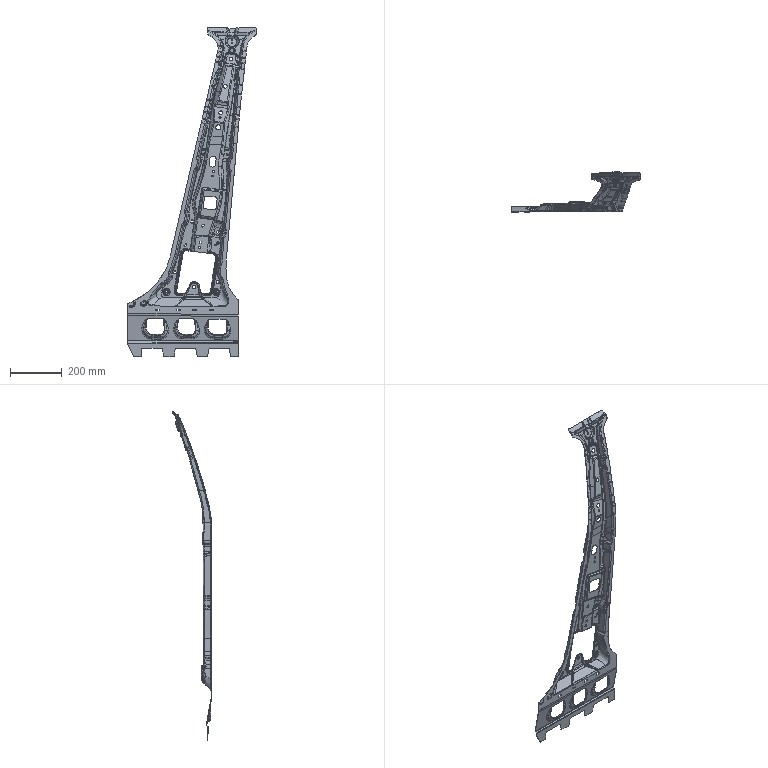Part | STEP file | FNA5401511 | 1 solid | 2335 faces | box 496.598 x 154.254 x 1271 mm | volume 355104 mm3 | spline 1559 | cylinder 448 | plane 222 | other 80 | sphere 26 | commonest cylinder face diameters 8 x65 10 x51 7.6 x39 10.4 x37 6 x24 30 x23